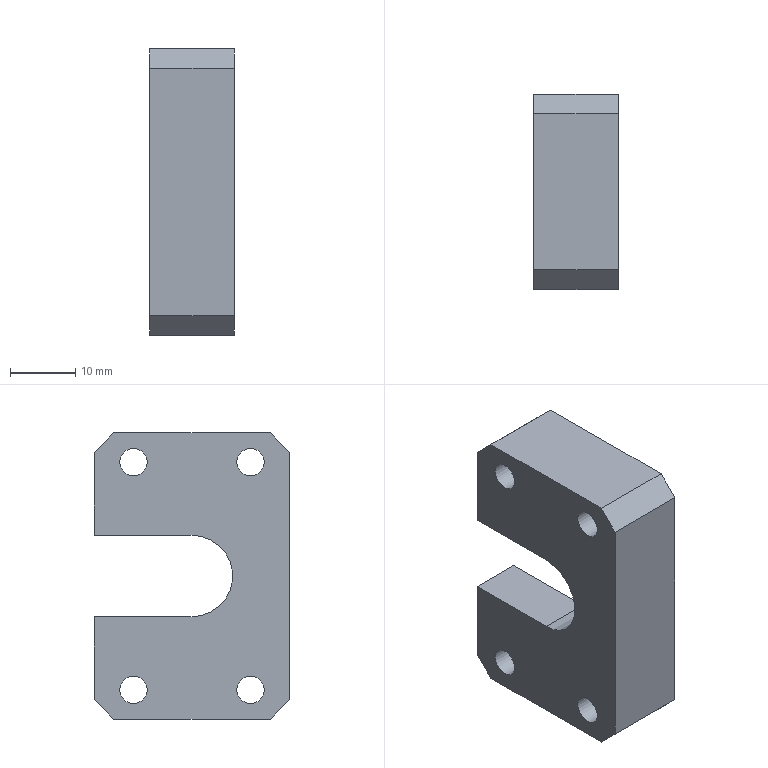Part | NX | 1 solid | 22 faces | box 13 x 30 x 44 mm | volume 11451 mm3 | plane 16 | cylinder 6 | commonest cylinder face diameters 4.2 x4 12.5 x1 23 x1
STEP:
#1=CARTESIAN_POINT('',(8.,0.,-6.25));
#2=VERTEX_POINT('',#1);
#3=CARTESIAN_POINT('',(8.,0.,6.25));
#4=VERTEX_POINT('',#3);
#5=CARTESIAN_POINT('',(8.,0.,0.));
#6=DIRECTION('',(1.,0.,0.));
#7=DIRECTION('',(0.,0.,-1.));
#8=AXIS2_PLACEMENT_3D('',#5,#6,#7);
#9=CIRCLE('',#8,6.25);
#10=EDGE_CURVE('',#2,#4,#9,.F.);
#11=ORIENTED_EDGE('',*,*,#10,.F.);
#12=CARTESIAN_POINT('',(0.,0.,-6.25));
#13=VERTEX_POINT('',#12);
#14=CARTESIAN_POINT('',(-7.,0.,-6.25));
#15=DIRECTION('',(1.,0.,0.));
#16=VECTOR('',#15,1000.);
#17=LINE('',#14,#16);
#18=EDGE_CURVE('',#13,#2,#17,.T.);
#19=ORIENTED_EDGE('',*,*,#18,.F.);
#20=CARTESIAN_POINT('',(0.,0.,6.25));
#21=VERTEX_POINT('',#20);
#22=CARTESIAN_POINT('',(0.,0.,0.));
#23=DIRECTION('',(1.,0.,0.));
#24=DIRECTION('',(0.,0.,-1.));
#25=AXIS2_PLACEMENT_3D('',#22,#23,#24);
#26=CIRCLE('',#25,6.25);
#27=EDGE_CURVE('',#21,#13,#26,.T.);
#28=ORIENTED_EDGE('',*,*,#27,.F.);
#29=CARTESIAN_POINT('',(-7.,0.,6.25));
#30=DIRECTION('',(1.,0.,0.));
#31=VECTOR('',#30,1000.);
#32=LINE('',#29,#31);
#33=EDGE_CURVE('',#21,#4,#32,.T.);
#34=ORIENTED_EDGE('',*,*,#33,.T.);
#35=EDGE_LOOP('',(#11,#19,#28,#34));
#36=FACE_BOUND('',#35,.T.);
#37=CARTESIAN_POINT('',(-7.,0.,0.));
#38=DIRECTION('',(1.,0.,0.));
#39=DIRECTION('',(0.,0.,-1.));
#40=AXIS2_PLACEMENT_3D('',#37,#38,#39);
#41=CYLINDRICAL_SURFACE('',#40,6.25);
#42=ADVANCED_FACE('',(#36),#41,.F.);
#43=CARTESIAN_POINT('',(8.,15.,6.25));
#44=VERTEX_POINT('',#43);
#45=CARTESIAN_POINT('',(8.,0.,6.25));
#46=DIRECTION('',(0.,1.,0.));
#47=VECTOR('',#46,1000.);
#48=LINE('',#45,#47);
#49=EDGE_CURVE('',#4,#44,#48,.T.);
#50=ORIENTED_EDGE('',*,*,#49,.F.);
#51=ORIENTED_EDGE('',*,*,#33,.F.);
#52=CARTESIAN_POINT('',(0.,15.,6.25));
#53=VERTEX_POINT('',#52);
#54=CARTESIAN_POINT('',(0.,0.,6.25));
#55=DIRECTION('',(0.,-1.,0.));
#56=VECTOR('',#55,1000.);
#57=LINE('',#54,#56);
#58=EDGE_CURVE('',#53,#21,#57,.T.);
#59=ORIENTED_EDGE('',*,*,#58,.F.);
#60=CARTESIAN_POINT('',(-7.,15.,6.25));
#61=DIRECTION('',(1.,0.,0.));
#62=VECTOR('',#61,1000.);
#63=LINE('',#60,#62);
#64=EDGE_CURVE('',#53,#44,#63,.T.);
#65=ORIENTED_EDGE('',*,*,#64,.T.);
#66=EDGE_LOOP('',(#50,#51,#59,#65));
#67=FACE_BOUND('',#66,.T.);
#68=CARTESIAN_POINT('',(-7.,0.,6.25));
#69=DIRECTION('',(0.,0.,1.));
#70=DIRECTION('',(1.,0.,0.));
#71=AXIS2_PLACEMENT_3D('',#68,#69,#70);
#72=PLANE('',#71);
#73=ADVANCED_FACE('',(#67),#72,.F.);
#74=CARTESIAN_POINT('',(8.,15.,-6.25));
#75=VERTEX_POINT('',#74);
#76=CARTESIAN_POINT('',(8.,0.,-6.25));
#77=DIRECTION('',(0.,-1.,0.));
#78=VECTOR('',#77,1000.);
#79=LINE('',#76,#78);
#80=EDGE_CURVE('',#75,#2,#79,.T.);
#81=ORIENTED_EDGE('',*,*,#80,.F.);
#82=CARTESIAN_POINT('',(0.,15.,-6.25));
#83=VERTEX_POINT('',#82);
#84=CARTESIAN_POINT('',(-7.,15.,-6.25));
#85=DIRECTION('',(1.,0.,0.));
#86=VECTOR('',#85,1000.);
#87=LINE('',#84,#86);
#88=EDGE_CURVE('',#83,#75,#87,.T.);
#89=ORIENTED_EDGE('',*,*,#88,.F.);
#90=CARTESIAN_POINT('',(0.,0.,-6.25));
#91=DIRECTION('',(0.,1.,0.));
#92=VECTOR('',#91,1000.);
#93=LINE('',#90,#92);
#94=EDGE_CURVE('',#13,#83,#93,.T.);
#95=ORIENTED_EDGE('',*,*,#94,.F.);
#96=ORIENTED_EDGE('',*,*,#18,.T.);
#97=EDGE_LOOP('',(#81,#89,#95,#96));
#98=FACE_BOUND('',#97,.T.);
#99=CARTESIAN_POINT('',(-7.,0.,-6.25));
#100=DIRECTION('',(0.,0.,-1.));
#101=DIRECTION('',(-1.,0.,0.));
#102=AXIS2_PLACEMENT_3D('',#99,#100,#101);
#103=PLANE('',#102);
#104=ADVANCED_FACE('',(#98),#103,.F.);
#105=CARTESIAN_POINT('',(13.,15.,11.5));
#106=VERTEX_POINT('',#105);
#107=CARTESIAN_POINT('',(13.,15.,19.));
#108=VERTEX_POINT('',#107);
#109=CARTESIAN_POINT('',(13.,15.,22.));
#110=DIRECTION('',(0.,0.,1.));
#111=VECTOR('',#110,1000.);
#112=LINE('',#109,#111);
#113=EDGE_CURVE('',#106,#108,#112,.T.);
#114=ORIENTED_EDGE('',*,*,#113,.F.);
#115=CARTESIAN_POINT('',(8.,15.,11.5));
#116=VERTEX_POINT('',#115);
#117=CARTESIAN_POINT('',(8.,15.,11.5));
#118=DIRECTION('',(1.,0.,0.));
#119=VECTOR('',#118,1000.);
#120=LINE('',#117,#119);
#121=EDGE_CURVE('',#116,#106,#120,.T.);
#122=ORIENTED_EDGE('',*,*,#121,.F.);
#123=CARTESIAN_POINT('',(8.,15.,22.));
#124=DIRECTION('',(0.,0.,1.));
#125=VECTOR('',#124,1000.);
#126=LINE('',#123,#125);
#127=EDGE_CURVE('',#44,#116,#126,.T.);
#128=ORIENTED_EDGE('',*,*,#127,.F.);
#129=ORIENTED_EDGE('',*,*,#64,.F.);
#130=CARTESIAN_POINT('',(0.,15.,19.));
#131=VERTEX_POINT('',#130);
#132=CARTESIAN_POINT('',(0.,15.,22.));
#133=DIRECTION('',(0.,0.,1.));
#134=VECTOR('',#133,1000.);
#135=LINE('',#132,#134);
#136=EDGE_CURVE('',#53,#131,#135,.T.);
#137=ORIENTED_EDGE('',*,*,#136,.T.);
#138=CARTESIAN_POINT('',(13.,15.,19.));
#139=DIRECTION('',(1.,0.,0.));
#140=VECTOR('',#139,1000.);
#141=LINE('',#138,#140);
#142=EDGE_CURVE('',#131,#108,#141,.T.);
#143=ORIENTED_EDGE('',*,*,#142,.T.);
#144=EDGE_LOOP('',(#114,#122,#128,#129,#137,#143));
#145=FACE_BOUND('',#144,.T.);
#146=CARTESIAN_POINT('',(13.,15.,22.));
#147=DIRECTION('',(0.,-1.,0.));
#148=DIRECTION('',(0.,0.,-1.));
#149=AXIS2_PLACEMENT_3D('',#146,#147,#148);
#150=PLANE('',#149);
#151=ADVANCED_FACE('',(#145),#150,.F.);
#152=CARTESIAN_POINT('',(0.,-12.,-22.));
#153=VERTEX_POINT('',#152);
#154=CARTESIAN_POINT('',(0.,12.,-22.));
#155=VERTEX_POINT('',#154);
#156=CARTESIAN_POINT('',(0.,15.,-22.));
#157=DIRECTION('',(0.,1.,0.));
#158=VECTOR('',#157,1000.);
#159=LINE('',#156,#158);
#160=EDGE_CURVE('',#153,#155,#159,.T.);
#161=ORIENTED_EDGE('',*,*,#160,.T.);
#162=CARTESIAN_POINT('',(13.,12.,-22.));
#163=VERTEX_POINT('',#162);
#164=CARTESIAN_POINT('',(13.,12.,-22.));
#165=DIRECTION('',(1.,0.,0.));
#166=VECTOR('',#165,1000.);
#167=LINE('',#164,#166);
#168=EDGE_CURVE('',#155,#163,#167,.T.);
#169=ORIENTED_EDGE('',*,*,#168,.T.);
#170=CARTESIAN_POINT('',(13.,-12.,-22.));
#171=VERTEX_POINT('',#170);
#172=CARTESIAN_POINT('',(13.,15.,-22.));
#173=DIRECTION('',(0.,1.,0.));
#174=VECTOR('',#173,1000.);
#175=LINE('',#172,#174);
#176=EDGE_CURVE('',#171,#163,#175,.T.);
#177=ORIENTED_EDGE('',*,*,#176,.F.);
#178=CARTESIAN_POINT('',(13.,-12.,-22.));
#179=DIRECTION('',(-1.,0.,0.));
#180=VECTOR('',#179,1000.);
#181=LINE('',#178,#180);
#182=EDGE_CURVE('',#171,#153,#181,.T.);
#183=ORIENTED_EDGE('',*,*,#182,.T.);
#184=EDGE_LOOP('',(#161,#169,#177,#183));
#185=FACE_BOUND('',#184,.T.);
#186=CARTESIAN_POINT('',(13.,15.,-22.));
#187=DIRECTION('',(0.,0.,1.));
#188=DIRECTION('',(0.,-1.,0.));
#189=AXIS2_PLACEMENT_3D('',#186,#187,#188);
#190=PLANE('',#189);
#191=ADVANCED_FACE('',(#185),#190,.F.);
#192=CARTESIAN_POINT('',(8.,15.,-11.5));
#193=VERTEX_POINT('',#192);
#194=CARTESIAN_POINT('',(8.,15.,22.));
#195=DIRECTION('',(0.,0.,1.));
#196=VECTOR('',#195,1000.);
#197=LINE('',#194,#196);
#198=EDGE_CURVE('',#193,#75,#197,.T.);
#199=ORIENTED_EDGE('',*,*,#198,.F.);
#200=CARTESIAN_POINT('',(13.,15.,-11.5));
#201=VERTEX_POINT('',#200);
#202=CARTESIAN_POINT('',(8.,15.,-11.5));
#203=DIRECTION('',(1.,0.,0.));
#204=VECTOR('',#203,1000.);
#205=LINE('',#202,#204);
#206=EDGE_CURVE('',#193,#201,#205,.T.);
#207=ORIENTED_EDGE('',*,*,#206,.T.);
#208=CARTESIAN_POINT('',(13.,15.,-19.));
#209=VERTEX_POINT('',#208);
#210=CARTESIAN_POINT('',(13.,15.,22.));
#211=DIRECTION('',(0.,0.,1.));
#212=VECTOR('',#211,1000.);
#213=LINE('',#210,#212);
#214=EDGE_CURVE('',#209,#201,#213,.T.);
#215=ORIENTED_EDGE('',*,*,#214,.F.);
#216=CARTESIAN_POINT('',(0.,15.,-19.));
#217=VERTEX_POINT('',#216);
#218=CARTESIAN_POINT('',(13.,15.,-19.));
#219=DIRECTION('',(-1.,0.,0.));
#220=VECTOR('',#219,1000.);
#221=LINE('',#218,#220);
#222=EDGE_CURVE('',#209,#217,#221,.T.);
#223=ORIENTED_EDGE('',*,*,#222,.T.);
#224=CARTESIAN_POINT('',(0.,15.,22.));
#225=DIRECTION('',(0.,0.,1.));
#226=VECTOR('',#225,1000.);
#227=LINE('',#224,#226);
#228=EDGE_CURVE('',#217,#83,#227,.T.);
#229=ORIENTED_EDGE('',*,*,#228,.T.);
#230=ORIENTED_EDGE('',*,*,#88,.T.);
#231=EDGE_LOOP('',(#199,#207,#215,#223,#229,#230));
#232=FACE_BOUND('',#231,.T.);
#233=CARTESIAN_POINT('',(13.,15.,22.));
#234=DIRECTION('',(0.,-1.,0.));
#235=DIRECTION('',(0.,0.,-1.));
#236=AXIS2_PLACEMENT_3D('',#233,#234,#235);
#237=PLANE('',#236);
#238=ADVANCED_FACE('',(#232),#237,.F.);
#239=CARTESIAN_POINT('',(13.,12.,22.));
#240=VERTEX_POINT('',#239);
#241=CARTESIAN_POINT('',(13.,-12.,22.));
#242=VERTEX_POINT('',#241);
#243=CARTESIAN_POINT('',(13.,15.,22.));
#244=DIRECTION('',(0.,-1.,0.));
#245=VECTOR('',#244,1000.);
#246=LINE('',#243,#245);
#247=EDGE_CURVE('',#240,#242,#246,.T.);
#248=ORIENTED_EDGE('',*,*,#247,.F.);
#249=CARTESIAN_POINT('',(0.,12.,22.));
#250=VERTEX_POINT('',#249);
#251=CARTESIAN_POINT('',(13.,12.,22.));
#252=DIRECTION('',(-1.,0.,0.));
#253=VECTOR('',#252,1000.);
#254=LINE('',#251,#253);
#255=EDGE_CURVE('',#240,#250,#254,.T.);
#256=ORIENTED_EDGE('',*,*,#255,.T.);
#257=CARTESIAN_POINT('',(0.,-12.,22.));
#258=VERTEX_POINT('',#257);
#259=CARTESIAN_POINT('',(0.,15.,22.));
#260=DIRECTION('',(0.,-1.,0.));
#261=VECTOR('',#260,1000.);
#262=LINE('',#259,#261);
#263=EDGE_CURVE('',#250,#258,#262,.T.);
#264=ORIENTED_EDGE('',*,*,#263,.T.);
#265=CARTESIAN_POINT('',(13.,-12.,22.));
#266=DIRECTION('',(1.,0.,0.));
#267=VECTOR('',#266,1000.);
#268=LINE('',#265,#267);
#269=EDGE_CURVE('',#258,#242,#268,.T.);
#270=ORIENTED_EDGE('',*,*,#269,.T.);
#271=EDGE_LOOP('',(#248,#256,#264,#270));
#272=FACE_BOUND('',#271,.T.);
#273=CARTESIAN_POINT('',(13.,15.,22.));
#274=DIRECTION('',(0.,0.,-1.));
#275=DIRECTION('',(0.,1.,0.));
#276=AXIS2_PLACEMENT_3D('',#273,#274,#275);
#277=PLANE('',#276);
#278=ADVANCED_FACE('',(#272),#277,.F.);
#279=CARTESIAN_POINT('',(13.,-15.,19.));
#280=VERTEX_POINT('',#279);
#281=CARTESIAN_POINT('',(13.,-15.,-19.));
#282=VERTEX_POINT('',#281);
#283=CARTESIAN_POINT('',(13.,-15.,22.));
#284=DIRECTION('',(0.,0.,-1.));
#285=VECTOR('',#284,1000.);
#286=LINE('',#283,#285);
#287=EDGE_CURVE('',#280,#282,#286,.T.);
#288=ORIENTED_EDGE('',*,*,#287,.F.);
#289=CARTESIAN_POINT('',(0.,-15.,19.));
#290=VERTEX_POINT('',#289);
#291=CARTESIAN_POINT('',(13.,-15.,19.));
#292=DIRECTION('',(-1.,0.,0.));
#293=VECTOR('',#292,1000.);
#294=LINE('',#291,#293);
#295=EDGE_CURVE('',#280,#290,#294,.T.);
#296=ORIENTED_EDGE('',*,*,#295,.T.);
#297=CARTESIAN_POINT('',(0.,-15.,-19.));
#298=VERTEX_POINT('',#297);
#299=CARTESIAN_POINT('',(0.,-15.,22.));
#300=DIRECTION('',(0.,0.,-1.));
#301=VECTOR('',#300,1000.);
#302=LINE('',#299,#301);
#303=EDGE_CURVE('',#290,#298,#302,.T.);
#304=ORIENTED_EDGE('',*,*,#303,.T.);
#305=CARTESIAN_POINT('',(13.,-15.,-19.));
#306=DIRECTION('',(1.,0.,0.));
#307=VECTOR('',#306,1000.);
#308=LINE('',#305,#307);
#309=EDGE_CURVE('',#298,#282,#308,.T.);
#310=ORIENTED_EDGE('',*,*,#309,.T.);
#311=EDGE_LOOP('',(#288,#296,#304,#310));
#312=FACE_BOUND('',#311,.T.);
#313=CARTESIAN_POINT('',(13.,-15.,22.));
#314=DIRECTION('',(0.,1.,0.));
#315=DIRECTION('',(0.,0.,1.));
#316=AXIS2_PLACEMENT_3D('',#313,#314,#315);
#317=PLANE('',#316);
#318=ADVANCED_FACE('',(#312),#317,.F.);
#319=CARTESIAN_POINT('',(13.,9.,-15.4));
#320=VERTEX_POINT('',#319);
#321=CARTESIAN_POINT('',(13.,9.,-17.5));
#322=DIRECTION('',(-1.,0.,0.));
#323=DIRECTION('',(0.,0.,1.));
#324=AXIS2_PLACEMENT_3D('',#321,#322,#323);
#325=CIRCLE('',#324,2.1);
#326=EDGE_CURVE('',#320,#320,#325,.T.);
#327=ORIENTED_EDGE('',*,*,#326,.T.);
#328=EDGE_LOOP('',(#327));
#329=FACE_BOUND('',#328,.T.);
#330=CARTESIAN_POINT('',(13.,-9.,-15.4));
#331=VERTEX_POINT('',#330);
#332=CARTESIAN_POINT('',(13.,-9.,-17.5));
#333=DIRECTION('',(-1.,0.,0.));
#334=DIRECTION('',(0.,0.,1.));
#335=AXIS2_PLACEMENT_3D('',#332,#333,#334);
#336=CIRCLE('',#335,2.1);
#337=EDGE_CURVE('',#331,#331,#336,.T.);
#338=ORIENTED_EDGE('',*,*,#337,.T.);
#339=EDGE_LOOP('',(#338));
#340=FACE_BOUND('',#339,.T.);
#341=CARTESIAN_POINT('',(13.,9.,19.6));
#342=VERTEX_POINT('',#341);
#343=CARTESIAN_POINT('',(13.,9.,17.5));
#344=DIRECTION('',(-1.,0.,0.));
#345=DIRECTION('',(0.,0.,1.));
#346=AXIS2_PLACEMENT_3D('',#343,#344,#345);
#347=CIRCLE('',#346,2.1);
#348=EDGE_CURVE('',#342,#342,#347,.T.);
#349=ORIENTED_EDGE('',*,*,#348,.T.);
#350=EDGE_LOOP('',(#349));
#351=FACE_BOUND('',#350,.T.);
#352=CARTESIAN_POINT('',(13.,-9.,19.6));
#353=VERTEX_POINT('',#352);
#354=CARTESIAN_POINT('',(13.,-9.,17.5));
#355=DIRECTION('',(-1.,0.,0.));
#356=DIRECTION('',(0.,0.,1.));
#357=AXIS2_PLACEMENT_3D('',#354,#355,#356);
#358=CIRCLE('',#357,2.1);
#359=EDGE_CURVE('',#353,#353,#358,.T.);
#360=ORIENTED_EDGE('',*,*,#359,.T.);
#361=EDGE_LOOP('',(#360));
#362=FACE_BOUND('',#361,.T.);
#363=CARTESIAN_POINT('',(13.,0.,11.5));
#364=VERTEX_POINT('',#363);
#365=CARTESIAN_POINT('',(13.,0.,11.5));
#366=DIRECTION('',(0.,-1.,0.));
#367=VECTOR('',#366,1000.);
#368=LINE('',#365,#367);
#369=EDGE_CURVE('',#106,#364,#368,.T.);
#370=ORIENTED_EDGE('',*,*,#369,.F.);
#371=ORIENTED_EDGE('',*,*,#113,.T.);
#372=CARTESIAN_POINT('',(13.,17.,17.));
#373=DIRECTION('',(0.,0.7071,-0.7071));
#374=VECTOR('',#373,1000.);
#375=LINE('',#372,#374);
#376=EDGE_CURVE('',#108,#240,#375,.F.);
#377=ORIENTED_EDGE('',*,*,#376,.T.);
#378=ORIENTED_EDGE('',*,*,#247,.T.);
#379=CARTESIAN_POINT('',(13.,-17.,17.));
#380=DIRECTION('',(0.,0.7071,0.7071));
#381=VECTOR('',#380,1000.);
#382=LINE('',#379,#381);
#383=EDGE_CURVE('',#242,#280,#382,.F.);
#384=ORIENTED_EDGE('',*,*,#383,.T.);
#385=ORIENTED_EDGE('',*,*,#287,.T.);
#386=CARTESIAN_POINT('',(13.,-17.,-17.));
#387=DIRECTION('',(0.,-0.7071,0.7071));
#388=VECTOR('',#387,1000.);
#389=LINE('',#386,#388);
#390=EDGE_CURVE('',#282,#171,#389,.F.);
#391=ORIENTED_EDGE('',*,*,#390,.T.);
#392=ORIENTED_EDGE('',*,*,#176,.T.);
#393=CARTESIAN_POINT('',(13.,17.,-17.));
#394=DIRECTION('',(0.,-0.7071,-0.7071));
#395=VECTOR('',#394,1000.);
#396=LINE('',#393,#395);
#397=EDGE_CURVE('',#163,#209,#396,.F.);
#398=ORIENTED_EDGE('',*,*,#397,.T.);
#399=ORIENTED_EDGE('',*,*,#214,.T.);
#400=CARTESIAN_POINT('',(13.,0.,-11.5));
#401=VERTEX_POINT('',#400);
#402=CARTESIAN_POINT('',(13.,0.,-11.5));
#403=DIRECTION('',(0.,1.,0.));
#404=VECTOR('',#403,1000.);
#405=LINE('',#402,#404);
#406=EDGE_CURVE('',#401,#201,#405,.T.);
#407=ORIENTED_EDGE('',*,*,#406,.F.);
#408=CARTESIAN_POINT('',(13.,0.,0.));
#409=DIRECTION('',(1.,0.,0.));
#410=DIRECTION('',(0.,0.,-1.));
#411=AXIS2_PLACEMENT_3D('',#408,#409,#410);
#412=CIRCLE('',#411,11.5);
#413=EDGE_CURVE('',#364,#401,#412,.T.);
#414=ORIENTED_EDGE('',*,*,#413,.F.);
#415=EDGE_LOOP('',(#370,#371,#377,#378,#384,#385,#391,#392,#398,#399,#407,#414));
#416=FACE_BOUND('',#415,.T.);
#417=CARTESIAN_POINT('',(13.,0.,0.));
#418=DIRECTION('',(1.,0.,0.));
#419=DIRECTION('',(0.,0.,-1.));
#420=AXIS2_PLACEMENT_3D('',#417,#418,#419);
#421=PLANE('',#420);
#422=ADVANCED_FACE('',(#329,#340,#351,#362,#416),#421,.T.);
#423=CARTESIAN_POINT('',(0.,9.,-15.4));
#424=VERTEX_POINT('',#423);
#425=CARTESIAN_POINT('',(0.,9.,-17.5));
#426=DIRECTION('',(-1.,0.,0.));
#427=DIRECTION('',(0.,0.,1.));
#428=AXIS2_PLACEMENT_3D('',#425,#426,#427);
#429=CIRCLE('',#428,2.1);
#430=EDGE_CURVE('',#424,#424,#429,.T.);
#431=ORIENTED_EDGE('',*,*,#430,.F.);
#432=EDGE_LOOP('',(#431));
#433=FACE_BOUND('',#432,.T.);
#434=CARTESIAN_POINT('',(0.,-9.,-15.4));
#435=VERTEX_POINT('',#434);
#436=CARTESIAN_POINT('',(0.,-9.,-17.5));
#437=DIRECTION('',(-1.,0.,0.));
#438=DIRECTION('',(0.,0.,1.));
#439=AXIS2_PLACEMENT_3D('',#436,#437,#438);
#440=CIRCLE('',#439,2.1);
#441=EDGE_CURVE('',#435,#435,#440,.T.);
#442=ORIENTED_EDGE('',*,*,#441,.F.);
#443=EDGE_LOOP('',(#442));
#444=FACE_BOUND('',#443,.T.);
#445=CARTESIAN_POINT('',(0.,9.,19.6));
#446=VERTEX_POINT('',#445);
#447=CARTESIAN_POINT('',(0.,9.,17.5));
#448=DIRECTION('',(-1.,0.,0.));
#449=DIRECTION('',(0.,0.,1.));
#450=AXIS2_PLACEMENT_3D('',#447,#448,#449);
#451=CIRCLE('',#450,2.1);
#452=EDGE_CURVE('',#446,#446,#451,.T.);
#453=ORIENTED_EDGE('',*,*,#452,.F.);
#454=EDGE_LOOP('',(#453));
#455=FACE_BOUND('',#454,.T.);
#456=CARTESIAN_POINT('',(0.,-9.,19.6));
#457=VERTEX_POINT('',#456);
#458=CARTESIAN_POINT('',(0.,-9.,17.5));
#459=DIRECTION('',(-1.,0.,0.));
#460=DIRECTION('',(0.,0.,1.));
#461=AXIS2_PLACEMENT_3D('',#458,#459,#460);
#462=CIRCLE('',#461,2.1);
#463=EDGE_CURVE('',#457,#457,#462,.T.);
#464=ORIENTED_EDGE('',*,*,#463,.F.);
#465=EDGE_LOOP('',(#464));
#466=FACE_BOUND('',#465,.T.);
#467=ORIENTED_EDGE('',*,*,#228,.F.);
#468=CARTESIAN_POINT('',(0.,15.,-19.));
#469=DIRECTION('',(0.,0.7071,0.7071));
#470=VECTOR('',#469,1000.);
#471=LINE('',#468,#470);
#472=EDGE_CURVE('',#217,#155,#471,.F.);
#473=ORIENTED_EDGE('',*,*,#472,.T.);
#474=ORIENTED_EDGE('',*,*,#160,.F.);
#475=CARTESIAN_POINT('',(0.,-12.,-22.));
#476=DIRECTION('',(0.,0.7071,-0.7071));
#477=VECTOR('',#476,1000.);
#478=LINE('',#475,#477);
#479=EDGE_CURVE('',#153,#298,#478,.F.);
#480=ORIENTED_EDGE('',*,*,#479,.T.);
#481=ORIENTED_EDGE('',*,*,#303,.F.);
#482=CARTESIAN_POINT('',(0.,-15.,19.));
#483=DIRECTION('',(0.,-0.7071,-0.7071));
#484=VECTOR('',#483,1000.);
#485=LINE('',#482,#484);
#486=EDGE_CURVE('',#290,#258,#485,.F.);
#487=ORIENTED_EDGE('',*,*,#486,.T.);
#488=ORIENTED_EDGE('',*,*,#263,.F.);
#489=CARTESIAN_POINT('',(0.,12.,22.));
#490=DIRECTION('',(0.,-0.7071,0.7071));
#491=VECTOR('',#490,1000.);
#492=LINE('',#489,#491);
#493=EDGE_CURVE('',#250,#131,#492,.F.);
#494=ORIENTED_EDGE('',*,*,#493,.T.);
#495=ORIENTED_EDGE('',*,*,#136,.F.);
#496=ORIENTED_EDGE('',*,*,#58,.T.);
#497=ORIENTED_EDGE('',*,*,#27,.T.);
#498=ORIENTED_EDGE('',*,*,#94,.T.);
#499=EDGE_LOOP('',(#467,#473,#474,#480,#481,#487,#488,#494,#495,#496,#497,#498));
#500=FACE_BOUND('',#499,.T.);
#501=CARTESIAN_POINT('',(0.,0.,0.));
#502=DIRECTION('',(1.,0.,0.));
#503=DIRECTION('',(0.,0.,-1.));
#504=AXIS2_PLACEMENT_3D('',#501,#502,#503);
#505=PLANE('',#504);
#506=ADVANCED_FACE('',(#433,#444,#455,#466,#500),#505,.F.);
#507=ORIENTED_EDGE('',*,*,#397,.F.);
#508=ORIENTED_EDGE('',*,*,#168,.F.);
#509=ORIENTED_EDGE('',*,*,#472,.F.);
#510=ORIENTED_EDGE('',*,*,#222,.F.);
#511=EDGE_LOOP('',(#507,#508,#509,#510));
#512=FACE_BOUND('',#511,.T.);
#513=CARTESIAN_POINT('',(13.,15.,-19.));
#514=DIRECTION('',(0.,-0.7071,0.7071));
#515=DIRECTION('',(-1.,0.,0.));
#516=AXIS2_PLACEMENT_3D('',#513,#514,#515);
#517=PLANE('',#516);
#518=ADVANCED_FACE('',(#512),#517,.F.);
#519=ORIENTED_EDGE('',*,*,#376,.F.);
#520=ORIENTED_EDGE('',*,*,#142,.F.);
#521=ORIENTED_EDGE('',*,*,#493,.F.);
#522=ORIENTED_EDGE('',*,*,#255,.F.);
#523=EDGE_LOOP('',(#519,#520,#521,#522));
#524=FACE_BOUND('',#523,.T.);
#525=CARTESIAN_POINT('',(13.,12.,22.));
#526=DIRECTION('',(0.,-0.7071,-0.7071));
#527=DIRECTION('',(-1.,0.,0.));
#528=AXIS2_PLACEMENT_3D('',#525,#526,#527);
#529=PLANE('',#528);
#530=ADVANCED_FACE('',(#524),#529,.F.);
#531=ORIENTED_EDGE('',*,*,#383,.F.);
#532=ORIENTED_EDGE('',*,*,#269,.F.);
#533=ORIENTED_EDGE('',*,*,#486,.F.);
#534=ORIENTED_EDGE('',*,*,#295,.F.);
#535=EDGE_LOOP('',(#531,#532,#533,#534));
#536=FACE_BOUND('',#535,.T.);
#537=CARTESIAN_POINT('',(13.,-15.,19.));
#538=DIRECTION('',(0.,0.7071,-0.7071));
#539=DIRECTION('',(-1.,0.,0.));
#540=AXIS2_PLACEMENT_3D('',#537,#538,#539);
#541=PLANE('',#540);
#542=ADVANCED_FACE('',(#536),#541,.F.);
#543=ORIENTED_EDGE('',*,*,#390,.F.);
#544=ORIENTED_EDGE('',*,*,#309,.F.);
#545=ORIENTED_EDGE('',*,*,#479,.F.);
#546=ORIENTED_EDGE('',*,*,#182,.F.);
#547=EDGE_LOOP('',(#543,#544,#545,#546));
#548=FACE_BOUND('',#547,.T.);
#549=CARTESIAN_POINT('',(13.,-12.,-22.));
#550=DIRECTION('',(0.,0.7071,0.7071));
#551=DIRECTION('',(-1.,0.,0.));
#552=AXIS2_PLACEMENT_3D('',#549,#550,#551);
#553=PLANE('',#552);
#554=ADVANCED_FACE('',(#548),#553,.F.);
#555=ORIENTED_EDGE('',*,*,#127,.T.);
#556=CARTESIAN_POINT('',(8.,0.,11.5));
#557=VERTEX_POINT('',#556);
#558=CARTESIAN_POINT('',(8.,0.,11.5));
#559=DIRECTION('',(0.,-1.,0.));
#560=VECTOR('',#559,1000.);
#561=LINE('',#558,#560);
#562=EDGE_CURVE('',#116,#557,#561,.T.);
#563=ORIENTED_EDGE('',*,*,#562,.T.);
#564=CARTESIAN_POINT('',(8.,0.,-11.5));
#565=VERTEX_POINT('',#564);
#566=CARTESIAN_POINT('',(8.,0.,0.));
#567=DIRECTION('',(1.,0.,0.));
#568=DIRECTION('',(0.,0.,-1.));
#569=AXIS2_PLACEMENT_3D('',#566,#567,#568);
#570=CIRCLE('',#569,11.5);
#571=EDGE_CURVE('',#557,#565,#570,.T.);
#572=ORIENTED_EDGE('',*,*,#571,.T.);
#573=CARTESIAN_POINT('',(8.,0.,-11.5));
#574=DIRECTION('',(0.,1.,0.));
#575=VECTOR('',#574,1000.);
#576=LINE('',#573,#575);
#577=EDGE_CURVE('',#565,#193,#576,.T.);
#578=ORIENTED_EDGE('',*,*,#577,.T.);
#579=ORIENTED_EDGE('',*,*,#198,.T.);
#580=ORIENTED_EDGE('',*,*,#80,.T.);
#581=ORIENTED_EDGE('',*,*,#10,.T.);
#582=ORIENTED_EDGE('',*,*,#49,.T.);
#583=EDGE_LOOP('',(#555,#563,#572,#578,#579,#580,#581,#582));
#584=FACE_BOUND('',#583,.T.);
#585=CARTESIAN_POINT('',(8.,0.,0.));
#586=DIRECTION('',(1.,0.,0.));
#587=DIRECTION('',(0.,0.,-1.));
#588=AXIS2_PLACEMENT_3D('',#585,#586,#587);
#589=PLANE('',#588);
#590=ADVANCED_FACE('',(#584),#589,.T.);
#591=ORIENTED_EDGE('',*,*,#413,.T.);
#592=CARTESIAN_POINT('',(8.,0.,-11.5));
#593=DIRECTION('',(1.,0.,0.));
#594=VECTOR('',#593,1000.);
#595=LINE('',#592,#594);
#596=EDGE_CURVE('',#565,#401,#595,.T.);
#597=ORIENTED_EDGE('',*,*,#596,.F.);
#598=ORIENTED_EDGE('',*,*,#571,.F.);
#599=CARTESIAN_POINT('',(8.,0.,11.5));
#600=DIRECTION('',(1.,0.,0.));
#601=VECTOR('',#600,1000.);
#602=LINE('',#599,#601);
#603=EDGE_CURVE('',#557,#364,#602,.T.);
#604=ORIENTED_EDGE('',*,*,#603,.T.);
#605=EDGE_LOOP('',(#591,#597,#598,#604));
#606=FACE_BOUND('',#605,.T.);
#607=CARTESIAN_POINT('',(8.,0.,0.));
#608=DIRECTION('',(1.,0.,0.));
#609=DIRECTION('',(0.,0.,-1.));
#610=AXIS2_PLACEMENT_3D('',#607,#608,#609);
#611=CYLINDRICAL_SURFACE('',#610,11.5);
#612=ADVANCED_FACE('',(#606),#611,.F.);
#613=ORIENTED_EDGE('',*,*,#369,.T.);
#614=ORIENTED_EDGE('',*,*,#603,.F.);
#615=ORIENTED_EDGE('',*,*,#562,.F.);
#616=ORIENTED_EDGE('',*,*,#121,.T.);
#617=EDGE_LOOP('',(#613,#614,#615,#616));
#618=FACE_BOUND('',#617,.T.);
#619=CARTESIAN_POINT('',(8.,0.,11.5));
#620=DIRECTION('',(0.,0.,1.));
#621=DIRECTION('',(1.,0.,0.));
#622=AXIS2_PLACEMENT_3D('',#619,#620,#621);
#623=PLANE('',#622);
#624=ADVANCED_FACE('',(#618),#623,.F.);
#625=ORIENTED_EDGE('',*,*,#406,.T.);
#626=ORIENTED_EDGE('',*,*,#206,.F.);
#627=ORIENTED_EDGE('',*,*,#577,.F.);
#628=ORIENTED_EDGE('',*,*,#596,.T.);
#629=EDGE_LOOP('',(#625,#626,#627,#628));
#630=FACE_BOUND('',#629,.T.);
#631=CARTESIAN_POINT('',(8.,0.,-11.5));
#632=DIRECTION('',(0.,0.,-1.));
#633=DIRECTION('',(-1.,0.,0.));
#634=AXIS2_PLACEMENT_3D('',#631,#632,#633);
#635=PLANE('',#634);
#636=ADVANCED_FACE('',(#630),#635,.F.);
#637=ORIENTED_EDGE('',*,*,#359,.F.);
#638=EDGE_LOOP('',(#637));
#639=FACE_BOUND('',#638,.T.);
#640=ORIENTED_EDGE('',*,*,#463,.T.);
#641=EDGE_LOOP('',(#640));
#642=FACE_BOUND('',#641,.T.);
#643=CARTESIAN_POINT('',(0.,-9.,17.5));
#644=DIRECTION('',(-1.,0.,0.));
#645=DIRECTION('',(0.,0.,1.));
#646=AXIS2_PLACEMENT_3D('',#643,#644,#645);
#647=CYLINDRICAL_SURFACE('',#646,2.1);
#648=ADVANCED_FACE('',(#639,#642),#647,.F.);
#649=ORIENTED_EDGE('',*,*,#348,.F.);
#650=EDGE_LOOP('',(#649));
#651=FACE_BOUND('',#650,.T.);
#652=ORIENTED_EDGE('',*,*,#452,.T.);
#653=EDGE_LOOP('',(#652));
#654=FACE_BOUND('',#653,.T.);
#655=CARTESIAN_POINT('',(0.,9.,17.5));
#656=DIRECTION('',(-1.,0.,0.));
#657=DIRECTION('',(0.,0.,1.));
#658=AXIS2_PLACEMENT_3D('',#655,#656,#657);
#659=CYLINDRICAL_SURFACE('',#658,2.1);
#660=ADVANCED_FACE('',(#651,#654),#659,.F.);
#661=ORIENTED_EDGE('',*,*,#337,.F.);
#662=EDGE_LOOP('',(#661));
#663=FACE_BOUND('',#662,.T.);
#664=ORIENTED_EDGE('',*,*,#441,.T.);
#665=EDGE_LOOP('',(#664));
#666=FACE_BOUND('',#665,.T.);
#667=CARTESIAN_POINT('',(0.,-9.,-17.5));
#668=DIRECTION('',(-1.,0.,0.));
#669=DIRECTION('',(0.,0.,1.));
#670=AXIS2_PLACEMENT_3D('',#667,#668,#669);
#671=CYLINDRICAL_SURFACE('',#670,2.1);
#672=ADVANCED_FACE('',(#663,#666),#671,.F.);
#673=ORIENTED_EDGE('',*,*,#326,.F.);
#674=EDGE_LOOP('',(#673));
#675=FACE_BOUND('',#674,.T.);
#676=ORIENTED_EDGE('',*,*,#430,.T.);
#677=EDGE_LOOP('',(#676));
#678=FACE_BOUND('',#677,.T.);
#679=CARTESIAN_POINT('',(0.,9.,-17.5));
#680=DIRECTION('',(-1.,0.,0.));
#681=DIRECTION('',(0.,0.,1.));
#682=AXIS2_PLACEMENT_3D('',#679,#680,#681);
#683=CYLINDRICAL_SURFACE('',#682,2.1);
#684=ADVANCED_FACE('',(#675,#678),#683,.F.);
#685=CLOSED_SHELL('',(#42,#73,#104,#151,#191,#238,#278,#318,#422,#506,#518,#530,#542,#554,#590,#612,#624,#636,#648,#660,#672,#684));
#686=MANIFOLD_SOLID_BREP('',#685);
#687=(LENGTH_UNIT()NAMED_UNIT(*)SI_UNIT(.MILLI.,.METRE.));
#688=UNCERTAINTY_MEASURE_WITH_UNIT(LENGTH_MEASURE(0.00001),#687,'','');
#689=(NAMED_UNIT(*)PLANE_ANGLE_UNIT()SI_UNIT($,.RADIAN.));
#690=(NAMED_UNIT(*)SI_UNIT($,.STERADIAN.)SOLID_ANGLE_UNIT());
#691=(GEOMETRIC_REPRESENTATION_CONTEXT(3)GLOBAL_UNCERTAINTY_ASSIGNED_CONTEXT((#688))GLOBAL_UNIT_ASSIGNED_CONTEXT((#687,#689,#690))REPRESENTATION_CONTEXT('',''));
#692=ADVANCED_BREP_SHAPE_REPRESENTATION('',(#686),#691);